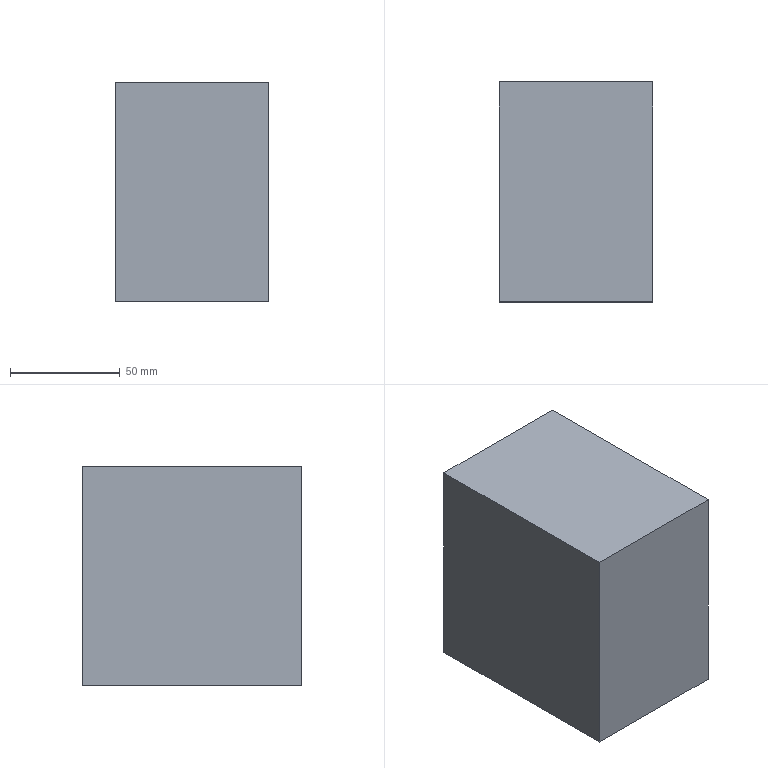Part | NX | features solid 2 | 1 solid | 6 faces | box 70 x 100 x 100 mm | volume 700000 mm3 | plane 6
STEP:
#1=CARTESIAN_POINT('',(1240.,-588.,-425.));
#2=VERTEX_POINT('',#1);
#3=CARTESIAN_POINT('',(1240.,-488.,-425.));
#4=VERTEX_POINT('',#3);
#5=CARTESIAN_POINT('',(1240.,-598.,-425.));
#6=DIRECTION('',(0.,1.,0.));
#7=VECTOR('',#6,1000.);
#8=LINE('',#5,#7);
#9=EDGE_CURVE('',#2,#4,#8,.T.);
#10=ORIENTED_EDGE('',*,*,#9,.F.);
#11=CARTESIAN_POINT('',(1170.,-588.,-425.));
#12=VERTEX_POINT('',#11);
#13=CARTESIAN_POINT('',(1170.,-588.,-425.));
#14=DIRECTION('',(1.,0.,0.));
#15=VECTOR('',#14,1000.);
#16=LINE('',#13,#15);
#17=EDGE_CURVE('',#12,#2,#16,.T.);
#18=ORIENTED_EDGE('',*,*,#17,.F.);
#19=CARTESIAN_POINT('',(1170.,-488.,-425.));
#20=VERTEX_POINT('',#19);
#21=CARTESIAN_POINT('',(1170.,-598.,-425.));
#22=DIRECTION('',(0.,1.,0.));
#23=VECTOR('',#22,1000.);
#24=LINE('',#21,#23);
#25=EDGE_CURVE('',#12,#20,#24,.T.);
#26=ORIENTED_EDGE('',*,*,#25,.T.);
#27=CARTESIAN_POINT('',(1170.,-488.,-425.));
#28=DIRECTION('',(1.,0.,0.));
#29=VECTOR('',#28,1000.);
#30=LINE('',#27,#29);
#31=EDGE_CURVE('',#20,#4,#30,.T.);
#32=ORIENTED_EDGE('',*,*,#31,.T.);
#33=EDGE_LOOP('',(#10,#18,#26,#32));
#34=FACE_BOUND('',#33,.T.);
#35=CARTESIAN_POINT('',(1170.,-598.,-425.));
#36=DIRECTION('',(0.,0.,-1.));
#37=DIRECTION('',(-1.,0.,0.));
#38=AXIS2_PLACEMENT_3D('',#35,#36,#37);
#39=PLANE('',#38);
#40=ADVANCED_FACE('',(#34),#39,.T.);
#41=CARTESIAN_POINT('',(1240.,-488.,-325.));
#42=VERTEX_POINT('',#41);
#43=CARTESIAN_POINT('',(1240.,-488.,-435.));
#44=DIRECTION('',(0.,0.,1.));
#45=VECTOR('',#44,1000.);
#46=LINE('',#43,#45);
#47=EDGE_CURVE('',#4,#42,#46,.T.);
#48=ORIENTED_EDGE('',*,*,#47,.F.);
#49=ORIENTED_EDGE('',*,*,#31,.F.);
#50=CARTESIAN_POINT('',(1170.,-488.,-325.));
#51=VERTEX_POINT('',#50);
#52=CARTESIAN_POINT('',(1170.,-488.,-435.));
#53=DIRECTION('',(0.,0.,1.));
#54=VECTOR('',#53,1000.);
#55=LINE('',#52,#54);
#56=EDGE_CURVE('',#20,#51,#55,.T.);
#57=ORIENTED_EDGE('',*,*,#56,.T.);
#58=CARTESIAN_POINT('',(1170.,-488.,-325.));
#59=DIRECTION('',(1.,0.,0.));
#60=VECTOR('',#59,1000.);
#61=LINE('',#58,#60);
#62=EDGE_CURVE('',#51,#42,#61,.T.);
#63=ORIENTED_EDGE('',*,*,#62,.T.);
#64=EDGE_LOOP('',(#48,#49,#57,#63));
#65=FACE_BOUND('',#64,.T.);
#66=CARTESIAN_POINT('',(1170.,-488.,-435.));
#67=DIRECTION('',(0.,1.,0.));
#68=DIRECTION('',(0.,0.,-1.));
#69=AXIS2_PLACEMENT_3D('',#66,#67,#68);
#70=PLANE('',#69);
#71=ADVANCED_FACE('',(#65),#70,.T.);
#72=CARTESIAN_POINT('',(1240.,-588.,-325.));
#73=VERTEX_POINT('',#72);
#74=CARTESIAN_POINT('',(1240.,-598.,-325.));
#75=DIRECTION('',(0.,1.,0.));
#76=VECTOR('',#75,1000.);
#77=LINE('',#74,#76);
#78=EDGE_CURVE('',#73,#42,#77,.T.);
#79=ORIENTED_EDGE('',*,*,#78,.T.);
#80=ORIENTED_EDGE('',*,*,#62,.F.);
#81=CARTESIAN_POINT('',(1170.,-588.,-325.));
#82=VERTEX_POINT('',#81);
#83=CARTESIAN_POINT('',(1170.,-598.,-325.));
#84=DIRECTION('',(0.,1.,0.));
#85=VECTOR('',#84,1000.);
#86=LINE('',#83,#85);
#87=EDGE_CURVE('',#82,#51,#86,.T.);
#88=ORIENTED_EDGE('',*,*,#87,.F.);
#89=CARTESIAN_POINT('',(1170.,-588.,-325.));
#90=DIRECTION('',(1.,0.,0.));
#91=VECTOR('',#90,1000.);
#92=LINE('',#89,#91);
#93=EDGE_CURVE('',#82,#73,#92,.T.);
#94=ORIENTED_EDGE('',*,*,#93,.T.);
#95=EDGE_LOOP('',(#79,#80,#88,#94));
#96=FACE_BOUND('',#95,.T.);
#97=CARTESIAN_POINT('',(1170.,-598.,-325.));
#98=DIRECTION('',(0.,0.,-1.));
#99=DIRECTION('',(-1.,0.,0.));
#100=AXIS2_PLACEMENT_3D('',#97,#98,#99);
#101=PLANE('',#100);
#102=ADVANCED_FACE('',(#96),#101,.F.);
#103=CARTESIAN_POINT('',(1240.,-588.,-435.));
#104=DIRECTION('',(0.,0.,1.));
#105=VECTOR('',#104,1000.);
#106=LINE('',#103,#105);
#107=EDGE_CURVE('',#2,#73,#106,.T.);
#108=ORIENTED_EDGE('',*,*,#107,.T.);
#109=ORIENTED_EDGE('',*,*,#93,.F.);
#110=CARTESIAN_POINT('',(1170.,-588.,-435.));
#111=DIRECTION('',(0.,0.,1.));
#112=VECTOR('',#111,1000.);
#113=LINE('',#110,#112);
#114=EDGE_CURVE('',#12,#82,#113,.T.);
#115=ORIENTED_EDGE('',*,*,#114,.F.);
#116=ORIENTED_EDGE('',*,*,#17,.T.);
#117=EDGE_LOOP('',(#108,#109,#115,#116));
#118=FACE_BOUND('',#117,.T.);
#119=CARTESIAN_POINT('',(1170.,-588.,-435.));
#120=DIRECTION('',(0.,1.,0.));
#121=DIRECTION('',(0.,0.,-1.));
#122=AXIS2_PLACEMENT_3D('',#119,#120,#121);
#123=PLANE('',#122);
#124=ADVANCED_FACE('',(#118),#123,.F.);
#125=ORIENTED_EDGE('',*,*,#25,.F.);
#126=ORIENTED_EDGE('',*,*,#114,.T.);
#127=ORIENTED_EDGE('',*,*,#87,.T.);
#128=ORIENTED_EDGE('',*,*,#56,.F.);
#129=EDGE_LOOP('',(#125,#126,#127,#128));
#130=FACE_BOUND('',#129,.T.);
#131=CARTESIAN_POINT('',(1170.,-598.,-435.));
#132=DIRECTION('',(1.,0.,0.));
#133=DIRECTION('',(0.,0.,-1.));
#134=AXIS2_PLACEMENT_3D('',#131,#132,#133);
#135=PLANE('',#134);
#136=ADVANCED_FACE('',(#130),#135,.F.);
#137=ORIENTED_EDGE('',*,*,#9,.T.);
#138=ORIENTED_EDGE('',*,*,#47,.T.);
#139=ORIENTED_EDGE('',*,*,#78,.F.);
#140=ORIENTED_EDGE('',*,*,#107,.F.);
#141=EDGE_LOOP('',(#137,#138,#139,#140));
#142=FACE_BOUND('',#141,.T.);
#143=CARTESIAN_POINT('',(1240.,-598.,-435.));
#144=DIRECTION('',(1.,0.,0.));
#145=DIRECTION('',(0.,0.,-1.));
#146=AXIS2_PLACEMENT_3D('',#143,#144,#145);
#147=PLANE('',#146);
#148=ADVANCED_FACE('',(#142),#147,.T.);
#149=CLOSED_SHELL('',(#40,#71,#102,#124,#136,#148));
#150=MANIFOLD_SOLID_BREP('',#149);
#151=(LENGTH_UNIT()NAMED_UNIT(*)SI_UNIT(.MILLI.,.METRE.));
#152=UNCERTAINTY_MEASURE_WITH_UNIT(LENGTH_MEASURE(0.00001),#151,'','');
#153=(NAMED_UNIT(*)PLANE_ANGLE_UNIT()SI_UNIT($,.RADIAN.));
#154=(NAMED_UNIT(*)SI_UNIT($,.STERADIAN.)SOLID_ANGLE_UNIT());
#155=(GEOMETRIC_REPRESENTATION_CONTEXT(3)GLOBAL_UNCERTAINTY_ASSIGNED_CONTEXT((#152))GLOBAL_UNIT_ASSIGNED_CONTEXT((#151,#153,#154))REPRESENTATION_CONTEXT('',''));
#156=ADVANCED_BREP_SHAPE_REPRESENTATION('',(#150),#155);